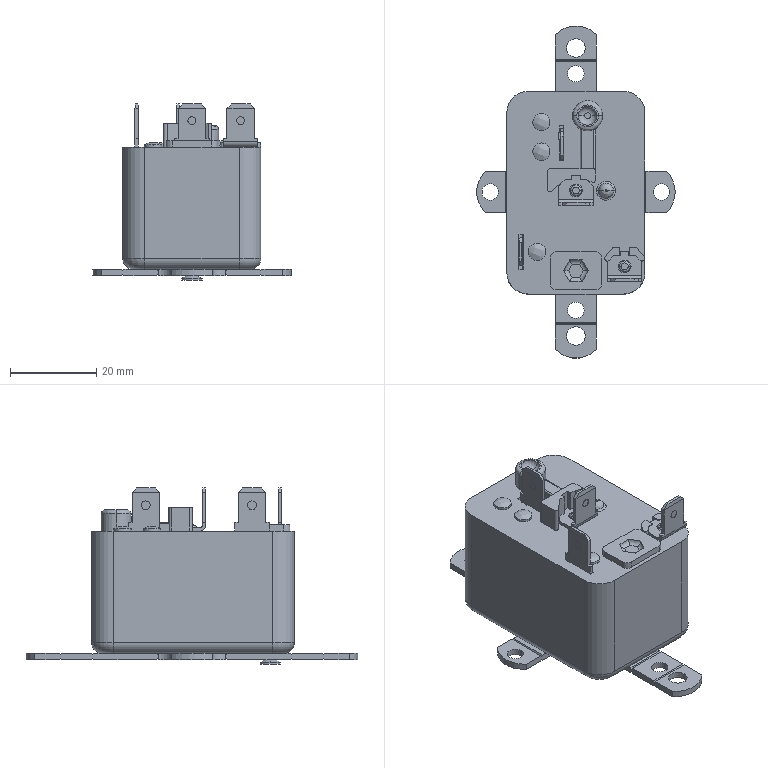Part | SolidWorks | features BaseBody 1 | 1 solid | 566 faces | box 46 x 77 x 40.798 mm | volume 41564 mm3 | plane 368 | cylinder 171 | spline 17 | torus 8 | cone 2 | commonest cylinder face diameters 2.5 x28 1 x25 2 x18 2.6 x15 3 x10 1.85 x8